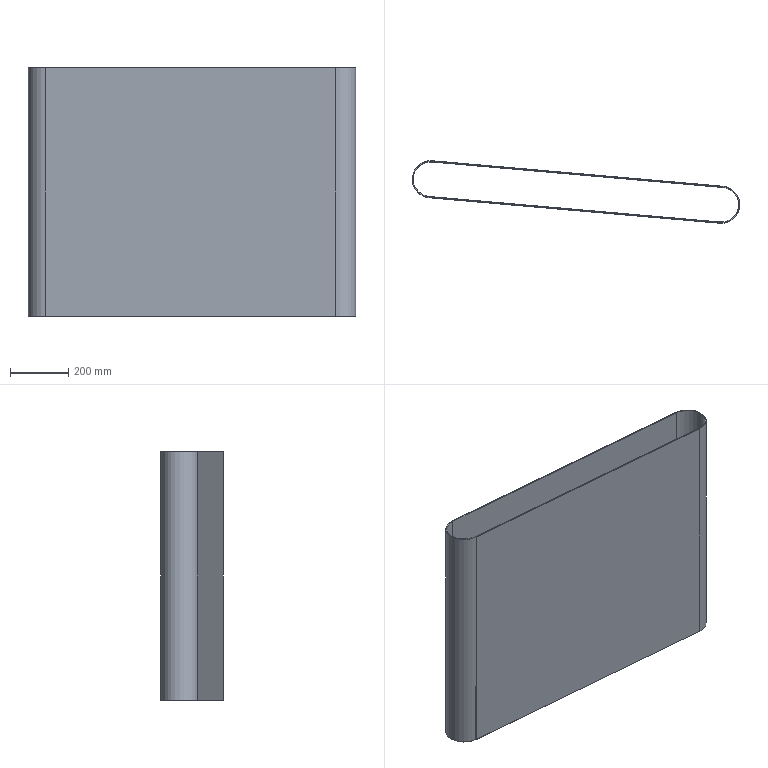Part | SolidWorks | features Extrusion 1 | 1 solid | 12 faces | box 1122 x 213.156 x 850 mm | volume 6085361 mm3 | cylinder 6 | plane 6 | commonest cylinder face diameters 120 x3 126 x3
STEP:
#1=CARTESIAN_POINT('',(3516.119,768.711,-425.));
#2=VERTEX_POINT('',#1);
#3=CARTESIAN_POINT('',(3570.89,708.939,-425.));
#4=VERTEX_POINT('',#3);
#5=CARTESIAN_POINT('',(3510.89,708.939,-425.));
#6=DIRECTION('',(0.,0.,-1.));
#7=DIRECTION('',(0.,-1.,0.));
#8=AXIS2_PLACEMENT_3D('',#5,#6,#7);
#9=CIRCLE('',#8,60.);
#10=EDGE_CURVE('',#2,#4,#9,.T.);
#11=ORIENTED_EDGE('',*,*,#10,.T.);
#12=CARTESIAN_POINT('',(3570.89,708.939,425.));
#13=VERTEX_POINT('',#12);
#14=CARTESIAN_POINT('',(3570.89,708.939,-1567.259));
#15=DIRECTION('',(0.,0.,1.));
#16=VECTOR('',#15,1000.);
#17=LINE('',#14,#16);
#18=EDGE_CURVE('',#4,#13,#17,.T.);
#19=ORIENTED_EDGE('',*,*,#18,.T.);
#20=CARTESIAN_POINT('',(3516.119,768.711,425.));
#21=VERTEX_POINT('',#20);
#22=CARTESIAN_POINT('',(3510.89,708.939,425.));
#23=DIRECTION('',(0.,0.,1.));
#24=DIRECTION('',(1.,0.,0.));
#25=AXIS2_PLACEMENT_3D('',#22,#23,#24);
#26=CIRCLE('',#25,60.);
#27=EDGE_CURVE('',#13,#21,#26,.T.);
#28=ORIENTED_EDGE('',*,*,#27,.T.);
#29=CARTESIAN_POINT('',(3516.119,768.711,-1567.259));
#30=DIRECTION('',(0.,0.,1.));
#31=VECTOR('',#30,1000.);
#32=LINE('',#29,#31);
#33=EDGE_CURVE('',#2,#21,#32,.T.);
#34=ORIENTED_EDGE('',*,*,#33,.F.);
#35=EDGE_LOOP('',(#11,#19,#28,#34));
#36=FACE_OUTER_BOUND('',#35,.T.);
#37=CARTESIAN_POINT('',(3510.89,708.939,-1567.259));
#38=DIRECTION('',(0.,0.,1.));
#39=DIRECTION('',(1.,0.,0.));
#40=AXIS2_PLACEMENT_3D('',#37,#38,#39);
#41=CYLINDRICAL_SURFACE('',#40,60.);
#42=ADVANCED_FACE('',(#36),#41,.F.);
#43=CARTESIAN_POINT('',(3573.89,708.939,-425.));
#44=VERTEX_POINT('',#43);
#45=CARTESIAN_POINT('',(3505.399,646.179,-425.));
#46=VERTEX_POINT('',#45);
#47=CARTESIAN_POINT('',(3510.89,708.939,-425.));
#48=DIRECTION('',(0.,0.,-1.));
#49=DIRECTION('',(0.,-1.,0.));
#50=AXIS2_PLACEMENT_3D('',#47,#48,#49);
#51=CIRCLE('',#50,63.);
#52=EDGE_CURVE('',#44,#46,#51,.T.);
#53=ORIENTED_EDGE('',*,*,#52,.F.);
#54=CARTESIAN_POINT('',(3573.89,708.939,425.));
#55=VERTEX_POINT('',#54);
#56=CARTESIAN_POINT('',(3573.89,708.939,-1567.259));
#57=DIRECTION('',(0.,0.,1.));
#58=VECTOR('',#57,1000.);
#59=LINE('',#56,#58);
#60=EDGE_CURVE('',#44,#55,#59,.T.);
#61=ORIENTED_EDGE('',*,*,#60,.T.);
#62=CARTESIAN_POINT('',(3505.399,646.179,425.));
#63=VERTEX_POINT('',#62);
#64=CARTESIAN_POINT('',(3510.89,708.939,425.));
#65=DIRECTION('',(0.,0.,1.));
#66=DIRECTION('',(1.,0.,0.));
#67=AXIS2_PLACEMENT_3D('',#64,#65,#66);
#68=CIRCLE('',#67,63.);
#69=EDGE_CURVE('',#63,#55,#68,.T.);
#70=ORIENTED_EDGE('',*,*,#69,.F.);
#71=CARTESIAN_POINT('',(3505.399,646.179,-1567.259));
#72=DIRECTION('',(0.,0.,1.));
#73=VECTOR('',#72,1000.);
#74=LINE('',#71,#73);
#75=EDGE_CURVE('',#46,#63,#74,.T.);
#76=ORIENTED_EDGE('',*,*,#75,.F.);
#77=EDGE_LOOP('',(#53,#61,#70,#76));
#78=FACE_OUTER_BOUND('',#77,.T.);
#79=CARTESIAN_POINT('',(3510.89,708.939,-1567.259));
#80=DIRECTION('',(0.,0.,1.));
#81=DIRECTION('',(1.,0.,0.));
#82=AXIS2_PLACEMENT_3D('',#79,#80,#81);
#83=CYLINDRICAL_SURFACE('',#82,63.);
#84=ADVANCED_FACE('',(#78),#83,.T.);
#85=CARTESIAN_POINT('',(2509.205,733.335,-425.));
#86=VERTEX_POINT('',#85);
#87=CARTESIAN_POINT('',(2509.205,733.335,-425.));
#88=DIRECTION('',(-0.9962,0.08716,0.));
#89=VECTOR('',#88,1000.);
#90=LINE('',#87,#89);
#91=EDGE_CURVE('',#46,#86,#90,.T.);
#92=ORIENTED_EDGE('',*,*,#91,.F.);
#93=ORIENTED_EDGE('',*,*,#75,.T.);
#94=CARTESIAN_POINT('',(2509.205,733.335,425.));
#95=VERTEX_POINT('',#94);
#96=CARTESIAN_POINT('',(2509.205,733.335,425.));
#97=DIRECTION('',(0.9962,-0.08716,0.));
#98=VECTOR('',#97,1000.);
#99=LINE('',#96,#98);
#100=EDGE_CURVE('',#95,#63,#99,.T.);
#101=ORIENTED_EDGE('',*,*,#100,.F.);
#102=CARTESIAN_POINT('',(2509.205,733.335,-1567.259));
#103=DIRECTION('',(0.,0.,1.));
#104=VECTOR('',#103,1000.);
#105=LINE('',#102,#104);
#106=EDGE_CURVE('',#86,#95,#105,.T.);
#107=ORIENTED_EDGE('',*,*,#106,.F.);
#108=EDGE_LOOP('',(#92,#93,#101,#107));
#109=FACE_OUTER_BOUND('',#108,.T.);
#110=CARTESIAN_POINT('',(2509.205,733.335,-1567.259));
#111=DIRECTION('',(-0.08716,-0.9962,0.));
#112=DIRECTION('',(0.9962,-0.08716,0.));
#113=AXIS2_PLACEMENT_3D('',#110,#111,#112);
#114=PLANE('',#113);
#115=ADVANCED_FACE('',(#109),#114,.T.);
#116=ORIENTED_EDGE('',*,*,#60,.F.);
#117=CARTESIAN_POINT('',(3516.381,771.7,-425.));
#118=VERTEX_POINT('',#117);
#119=CARTESIAN_POINT('',(3510.89,708.939,-425.));
#120=DIRECTION('',(0.,0.,-1.));
#121=DIRECTION('',(0.,-1.,0.));
#122=AXIS2_PLACEMENT_3D('',#119,#120,#121);
#123=CIRCLE('',#122,63.);
#124=EDGE_CURVE('',#118,#44,#123,.T.);
#125=ORIENTED_EDGE('',*,*,#124,.F.);
#126=CARTESIAN_POINT('',(3516.381,771.7,425.));
#127=VERTEX_POINT('',#126);
#128=CARTESIAN_POINT('',(3516.381,771.7,-1567.259));
#129=DIRECTION('',(0.,0.,1.));
#130=VECTOR('',#129,1000.);
#131=LINE('',#128,#130);
#132=EDGE_CURVE('',#118,#127,#131,.T.);
#133=ORIENTED_EDGE('',*,*,#132,.T.);
#134=CARTESIAN_POINT('',(3510.89,708.939,425.));
#135=DIRECTION('',(0.,0.,1.));
#136=DIRECTION('',(1.,0.,0.));
#137=AXIS2_PLACEMENT_3D('',#134,#135,#136);
#138=CIRCLE('',#137,63.);
#139=EDGE_CURVE('',#55,#127,#138,.T.);
#140=ORIENTED_EDGE('',*,*,#139,.F.);
#141=EDGE_LOOP('',(#116,#125,#133,#140));
#142=FACE_OUTER_BOUND('',#141,.T.);
#143=CARTESIAN_POINT('',(3510.89,708.939,-1567.259));
#144=DIRECTION('',(0.,0.,1.));
#145=DIRECTION('',(1.,0.,0.));
#146=AXIS2_PLACEMENT_3D('',#143,#144,#145);
#147=CYLINDRICAL_SURFACE('',#146,63.);
#148=ADVANCED_FACE('',(#142),#147,.T.);
#149=CARTESIAN_POINT('',(2520.186,858.855,-425.));
#150=VERTEX_POINT('',#149);
#151=CARTESIAN_POINT('',(2520.186,858.855,-425.));
#152=DIRECTION('',(0.9962,-0.08716,0.));
#153=VECTOR('',#152,1000.);
#154=LINE('',#151,#153);
#155=EDGE_CURVE('',#150,#118,#154,.T.);
#156=ORIENTED_EDGE('',*,*,#155,.F.);
#157=CARTESIAN_POINT('',(2520.186,858.855,425.));
#158=VERTEX_POINT('',#157);
#159=CARTESIAN_POINT('',(2520.186,858.855,-1567.259));
#160=DIRECTION('',(0.,0.,1.));
#161=VECTOR('',#160,1000.);
#162=LINE('',#159,#161);
#163=EDGE_CURVE('',#150,#158,#162,.T.);
#164=ORIENTED_EDGE('',*,*,#163,.T.);
#165=CARTESIAN_POINT('',(2520.186,858.855,425.));
#166=DIRECTION('',(-0.9962,0.08716,0.));
#167=VECTOR('',#166,1000.);
#168=LINE('',#165,#167);
#169=EDGE_CURVE('',#127,#158,#168,.T.);
#170=ORIENTED_EDGE('',*,*,#169,.F.);
#171=ORIENTED_EDGE('',*,*,#132,.F.);
#172=EDGE_LOOP('',(#156,#164,#170,#171));
#173=FACE_OUTER_BOUND('',#172,.T.);
#174=CARTESIAN_POINT('',(2520.186,858.855,-1567.259));
#175=DIRECTION('',(0.08716,0.9962,0.));
#176=DIRECTION('',(-0.9962,0.08716,0.));
#177=AXIS2_PLACEMENT_3D('',#174,#175,#176);
#178=PLANE('',#177);
#179=ADVANCED_FACE('',(#173),#178,.T.);
#180=CARTESIAN_POINT('',(2514.695,796.095,-425.));
#181=DIRECTION('',(0.,0.,-1.));
#182=DIRECTION('',(0.,-1.,0.));
#183=AXIS2_PLACEMENT_3D('',#180,#181,#182);
#184=CIRCLE('',#183,63.);
#185=EDGE_CURVE('',#86,#150,#184,.T.);
#186=ORIENTED_EDGE('',*,*,#185,.F.);
#187=ORIENTED_EDGE('',*,*,#106,.T.);
#188=CARTESIAN_POINT('',(2514.695,796.095,425.));
#189=DIRECTION('',(0.,0.,1.));
#190=DIRECTION('',(1.,0.,0.));
#191=AXIS2_PLACEMENT_3D('',#188,#189,#190);
#192=CIRCLE('',#191,63.);
#193=EDGE_CURVE('',#158,#95,#192,.T.);
#194=ORIENTED_EDGE('',*,*,#193,.F.);
#195=ORIENTED_EDGE('',*,*,#163,.F.);
#196=EDGE_LOOP('',(#186,#187,#194,#195));
#197=FACE_OUTER_BOUND('',#196,.T.);
#198=CARTESIAN_POINT('',(2514.695,796.095,-1567.259));
#199=DIRECTION('',(0.,0.,1.));
#200=DIRECTION('',(1.,0.,0.));
#201=AXIS2_PLACEMENT_3D('',#198,#199,#200);
#202=CYLINDRICAL_SURFACE('',#201,63.);
#203=ADVANCED_FACE('',(#197),#202,.T.);
#204=CARTESIAN_POINT('',(2519.925,855.867,425.));
#205=VERTEX_POINT('',#204);
#206=CARTESIAN_POINT('',(2509.466,736.324,425.));
#207=VERTEX_POINT('',#206);
#208=CARTESIAN_POINT('',(2514.695,796.095,425.));
#209=DIRECTION('',(0.,0.,1.));
#210=DIRECTION('',(1.,0.,0.));
#211=AXIS2_PLACEMENT_3D('',#208,#209,#210);
#212=CIRCLE('',#211,60.);
#213=EDGE_CURVE('',#205,#207,#212,.T.);
#214=ORIENTED_EDGE('',*,*,#213,.F.);
#215=CARTESIAN_POINT('',(2519.925,855.867,425.));
#216=DIRECTION('',(-0.9962,0.08716,0.));
#217=VECTOR('',#216,1000.);
#218=LINE('',#215,#217);
#219=EDGE_CURVE('',#21,#205,#218,.T.);
#220=ORIENTED_EDGE('',*,*,#219,.F.);
#221=ORIENTED_EDGE('',*,*,#27,.F.);
#222=CARTESIAN_POINT('',(3505.661,649.168,425.));
#223=VERTEX_POINT('',#222);
#224=CARTESIAN_POINT('',(3510.89,708.939,425.));
#225=DIRECTION('',(0.,0.,1.));
#226=DIRECTION('',(1.,0.,0.));
#227=AXIS2_PLACEMENT_3D('',#224,#225,#226);
#228=CIRCLE('',#227,60.);
#229=EDGE_CURVE('',#223,#13,#228,.T.);
#230=ORIENTED_EDGE('',*,*,#229,.F.);
#231=CARTESIAN_POINT('',(2509.466,736.324,425.));
#232=DIRECTION('',(0.9962,-0.08716,0.));
#233=VECTOR('',#232,1000.);
#234=LINE('',#231,#233);
#235=EDGE_CURVE('',#207,#223,#234,.T.);
#236=ORIENTED_EDGE('',*,*,#235,.F.);
#237=EDGE_LOOP('',(#214,#220,#221,#230,#236));
#238=FACE_BOUND('',#237,.T.);
#239=ORIENTED_EDGE('',*,*,#193,.T.);
#240=ORIENTED_EDGE('',*,*,#100,.T.);
#241=ORIENTED_EDGE('',*,*,#69,.T.);
#242=ORIENTED_EDGE('',*,*,#139,.T.);
#243=ORIENTED_EDGE('',*,*,#169,.T.);
#244=EDGE_LOOP('',(#239,#240,#241,#242,#243));
#245=FACE_OUTER_BOUND('',#244,.T.);
#246=CARTESIAN_POINT('',(2514.695,796.095,425.));
#247=DIRECTION('',(0.,0.,1.));
#248=DIRECTION('',(1.,0.,0.));
#249=AXIS2_PLACEMENT_3D('',#246,#247,#248);
#250=PLANE('',#249);
#251=ADVANCED_FACE('',(#238,#245),#250,.T.);
#252=CARTESIAN_POINT('',(3505.661,649.168,-425.));
#253=VERTEX_POINT('',#252);
#254=CARTESIAN_POINT('',(3505.661,649.168,-1567.259));
#255=DIRECTION('',(0.,0.,1.));
#256=VECTOR('',#255,1000.);
#257=LINE('',#254,#256);
#258=EDGE_CURVE('',#253,#223,#257,.T.);
#259=ORIENTED_EDGE('',*,*,#258,.F.);
#260=CARTESIAN_POINT('',(2509.466,736.324,-425.));
#261=VERTEX_POINT('',#260);
#262=CARTESIAN_POINT('',(2509.466,736.324,-425.));
#263=DIRECTION('',(-0.9962,0.08716,0.));
#264=VECTOR('',#263,1000.);
#265=LINE('',#262,#264);
#266=EDGE_CURVE('',#253,#261,#265,.T.);
#267=ORIENTED_EDGE('',*,*,#266,.T.);
#268=CARTESIAN_POINT('',(2509.466,736.324,-1567.259));
#269=DIRECTION('',(0.,0.,1.));
#270=VECTOR('',#269,1000.);
#271=LINE('',#268,#270);
#272=EDGE_CURVE('',#261,#207,#271,.T.);
#273=ORIENTED_EDGE('',*,*,#272,.T.);
#274=ORIENTED_EDGE('',*,*,#235,.T.);
#275=EDGE_LOOP('',(#259,#267,#273,#274));
#276=FACE_OUTER_BOUND('',#275,.T.);
#277=CARTESIAN_POINT('',(2509.466,736.324,-1567.259));
#278=DIRECTION('',(-0.08716,-0.9962,0.));
#279=DIRECTION('',(0.9962,-0.08716,0.));
#280=AXIS2_PLACEMENT_3D('',#277,#278,#279);
#281=PLANE('',#280);
#282=ADVANCED_FACE('',(#276),#281,.F.);
#283=ORIENTED_EDGE('',*,*,#18,.F.);
#284=CARTESIAN_POINT('',(3510.89,708.939,-425.));
#285=DIRECTION('',(0.,0.,-1.));
#286=DIRECTION('',(0.,-1.,0.));
#287=AXIS2_PLACEMENT_3D('',#284,#285,#286);
#288=CIRCLE('',#287,60.);
#289=EDGE_CURVE('',#4,#253,#288,.T.);
#290=ORIENTED_EDGE('',*,*,#289,.T.);
#291=ORIENTED_EDGE('',*,*,#258,.T.);
#292=ORIENTED_EDGE('',*,*,#229,.T.);
#293=EDGE_LOOP('',(#283,#290,#291,#292));
#294=FACE_OUTER_BOUND('',#293,.T.);
#295=CARTESIAN_POINT('',(3510.89,708.939,-1567.259));
#296=DIRECTION('',(0.,0.,1.));
#297=DIRECTION('',(1.,0.,0.));
#298=AXIS2_PLACEMENT_3D('',#295,#296,#297);
#299=CYLINDRICAL_SURFACE('',#298,60.);
#300=ADVANCED_FACE('',(#294),#299,.F.);
#301=CARTESIAN_POINT('',(2519.925,855.867,-425.));
#302=VERTEX_POINT('',#301);
#303=CARTESIAN_POINT('',(2519.925,855.867,-1567.259));
#304=DIRECTION('',(0.,0.,1.));
#305=VECTOR('',#304,1000.);
#306=LINE('',#303,#305);
#307=EDGE_CURVE('',#302,#205,#306,.T.);
#308=ORIENTED_EDGE('',*,*,#307,.F.);
#309=CARTESIAN_POINT('',(2519.925,855.867,-425.));
#310=DIRECTION('',(0.9962,-0.08716,0.));
#311=VECTOR('',#310,1000.);
#312=LINE('',#309,#311);
#313=EDGE_CURVE('',#302,#2,#312,.T.);
#314=ORIENTED_EDGE('',*,*,#313,.T.);
#315=ORIENTED_EDGE('',*,*,#33,.T.);
#316=ORIENTED_EDGE('',*,*,#219,.T.);
#317=EDGE_LOOP('',(#308,#314,#315,#316));
#318=FACE_OUTER_BOUND('',#317,.T.);
#319=CARTESIAN_POINT('',(2519.925,855.867,-1567.259));
#320=DIRECTION('',(0.08716,0.9962,0.));
#321=DIRECTION('',(-0.9962,0.08716,0.));
#322=AXIS2_PLACEMENT_3D('',#319,#320,#321);
#323=PLANE('',#322);
#324=ADVANCED_FACE('',(#318),#323,.F.);
#325=ORIENTED_EDGE('',*,*,#272,.F.);
#326=CARTESIAN_POINT('',(2514.695,796.095,-425.));
#327=DIRECTION('',(0.,0.,-1.));
#328=DIRECTION('',(0.,-1.,0.));
#329=AXIS2_PLACEMENT_3D('',#326,#327,#328);
#330=CIRCLE('',#329,60.);
#331=EDGE_CURVE('',#261,#302,#330,.T.);
#332=ORIENTED_EDGE('',*,*,#331,.T.);
#333=ORIENTED_EDGE('',*,*,#307,.T.);
#334=ORIENTED_EDGE('',*,*,#213,.T.);
#335=EDGE_LOOP('',(#325,#332,#333,#334));
#336=FACE_OUTER_BOUND('',#335,.T.);
#337=CARTESIAN_POINT('',(2514.695,796.095,-1567.259));
#338=DIRECTION('',(0.,0.,1.));
#339=DIRECTION('',(1.,0.,0.));
#340=AXIS2_PLACEMENT_3D('',#337,#338,#339);
#341=CYLINDRICAL_SURFACE('',#340,60.);
#342=ADVANCED_FACE('',(#336),#341,.F.);
#343=ORIENTED_EDGE('',*,*,#185,.T.);
#344=ORIENTED_EDGE('',*,*,#155,.T.);
#345=ORIENTED_EDGE('',*,*,#124,.T.);
#346=ORIENTED_EDGE('',*,*,#52,.T.);
#347=ORIENTED_EDGE('',*,*,#91,.T.);
#348=EDGE_LOOP('',(#343,#344,#345,#346,#347));
#349=FACE_OUTER_BOUND('',#348,.T.);
#350=ORIENTED_EDGE('',*,*,#266,.F.);
#351=ORIENTED_EDGE('',*,*,#289,.F.);
#352=ORIENTED_EDGE('',*,*,#10,.F.);
#353=ORIENTED_EDGE('',*,*,#313,.F.);
#354=ORIENTED_EDGE('',*,*,#331,.F.);
#355=EDGE_LOOP('',(#350,#351,#352,#353,#354));
#356=FACE_BOUND('',#355,.T.);
#357=CARTESIAN_POINT('',(3510.89,768.939,-425.));
#358=DIRECTION('',(0.,0.,1.));
#359=DIRECTION('',(1.,0.,0.));
#360=AXIS2_PLACEMENT_3D('',#357,#358,#359);
#361=PLANE('',#360);
#362=ADVANCED_FACE('',(#349,#356),#361,.F.);
#363=CLOSED_SHELL('',(#42,#84,#115,#148,#179,#203,#251,#282,#300,#324,#342,#362));
#364=MANIFOLD_SOLID_BREP('',#363);
#365=CARTESIAN_POINT('',(0.,0.,0.));
#366=DIRECTION('',(0.,0.,1.));
#367=DIRECTION('',(1.,0.,0.));
#368=AXIS2_PLACEMENT_3D('',#365,#366,#367);
#369=(LENGTH_UNIT()NAMED_UNIT(*)SI_UNIT(.MILLI.,.METRE.));
#370=UNCERTAINTY_MEASURE_WITH_UNIT(LENGTH_MEASURE(0.00001),#369,'','');
#371=(NAMED_UNIT(*)PLANE_ANGLE_UNIT()SI_UNIT($,.RADIAN.));
#372=(NAMED_UNIT(*)SI_UNIT($,.STERADIAN.)SOLID_ANGLE_UNIT());
#373=(GEOMETRIC_REPRESENTATION_CONTEXT(3)GLOBAL_UNCERTAINTY_ASSIGNED_CONTEXT((#370))GLOBAL_UNIT_ASSIGNED_CONTEXT((#369,#371,#372))REPRESENTATION_CONTEXT('',''));
#374=ADVANCED_BREP_SHAPE_REPRESENTATION('',(#364,#368),#373);